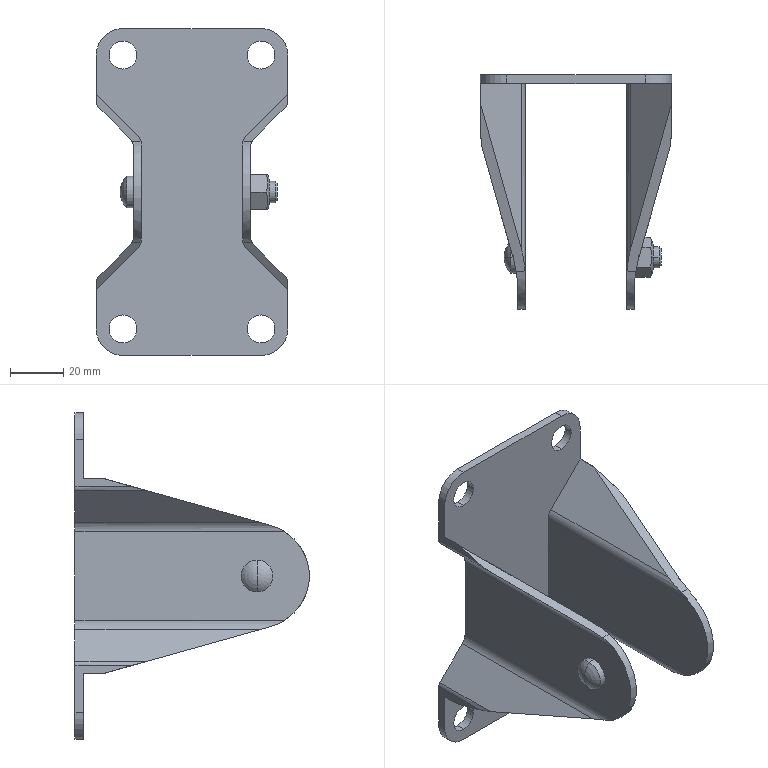Part | STEP file | SceondCKH75fixed | 1 solid | 71 faces | box 72 x 88.179 x 123 mm | volume 53019 mm3 | cylinder 34 | plane 31 | torus 4 | cone 2 | commonest cylinder face diameters 10 x8 10.5 x8 0.2 x4 4 x4 20 x4 8 x2